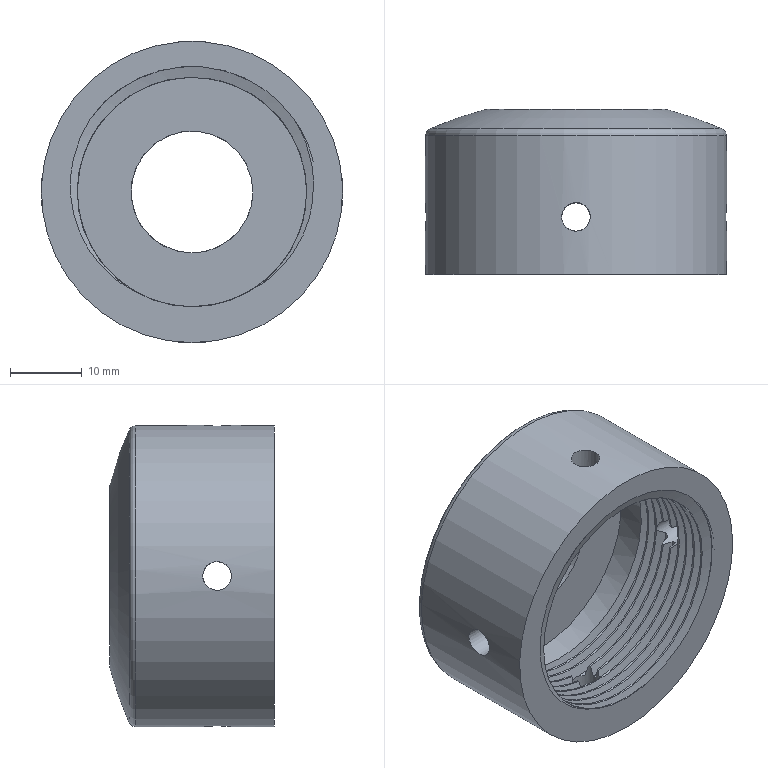Part | NX | features DATUM_CSYS 5, SKETCH 4, EXTRUDE 3, BLEND 1, SWP104 1, THREADS 1 | 1 solid | 57 faces | box 42 x 23 x 42 mm | volume 14105 mm3 | cylinder 30 | spline 21 | plane 4 | sphere 1 | torus 1 | commonest cylinder face diameters 32 x13 35 x11 4 x4 17 x1 42 x1